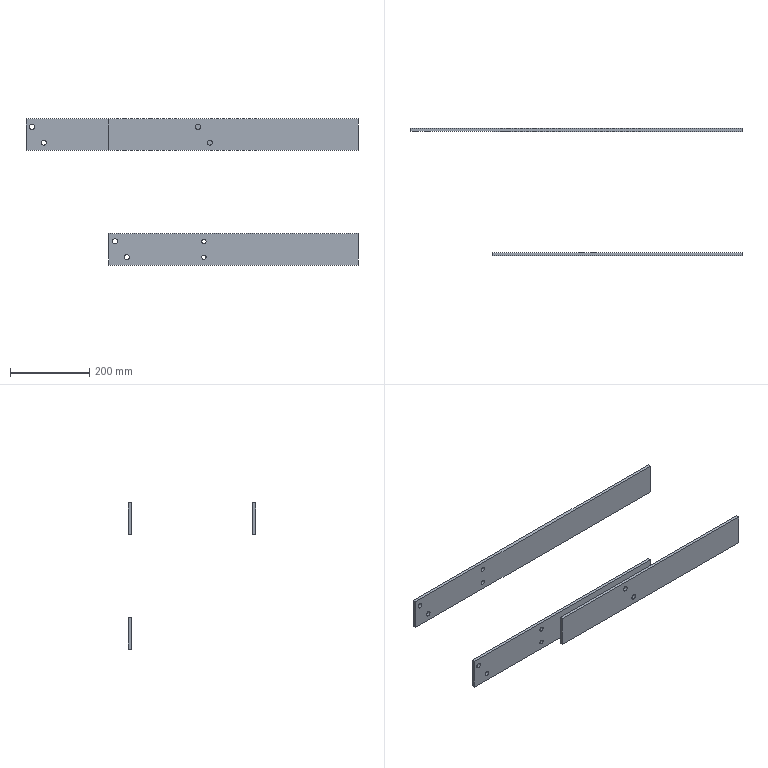Part | SolidWorks | features BaseBody 3 | 3 solids | 38 faces | box 840 x 323 x 370 mm | volume 1334588 mm3 | cylinder 20 | plane 18 | commonest cylinder face diameters 13 x12 11 x8
STEP:
#1=CARTESIAN_POINT('',(561.946,-3179.473,1586.471));
#2=VERTEX_POINT('',#1);
#3=CARTESIAN_POINT('',(561.946,-3179.473,1573.471));
#4=VERTEX_POINT('',#3);
#5=CARTESIAN_POINT('',(561.946,-3179.473,1579.971));
#6=DIRECTION('',(0.,-1.,0.));
#7=DIRECTION('',(0.,0.,-1.));
#8=AXIS2_PLACEMENT_3D('',#5,#6,#7);
#9=CIRCLE('',#8,6.5);
#10=EDGE_CURVE('',#2,#4,#9,.T.);
#11=ORIENTED_EDGE('',*,*,#10,.F.);
#12=CARTESIAN_POINT('',(561.946,-3187.473,1586.471));
#13=VERTEX_POINT('',#12);
#14=CARTESIAN_POINT('',(561.946,-3170.754,1586.471));
#15=DIRECTION('',(0.,-1.,0.));
#16=VECTOR('',#15,1000.);
#17=LINE('',#14,#16);
#18=EDGE_CURVE('',#2,#13,#17,.T.);
#19=ORIENTED_EDGE('',*,*,#18,.T.);
#20=CARTESIAN_POINT('',(561.946,-3187.473,1573.471));
#21=VERTEX_POINT('',#20);
#22=CARTESIAN_POINT('',(561.946,-3187.473,1579.971));
#23=DIRECTION('',(0.,1.,0.));
#24=DIRECTION('',(0.,0.,-1.));
#25=AXIS2_PLACEMENT_3D('',#22,#23,#24);
#26=CIRCLE('',#25,6.5);
#27=EDGE_CURVE('',#21,#13,#26,.T.);
#28=ORIENTED_EDGE('',*,*,#27,.F.);
#29=CARTESIAN_POINT('',(561.946,-3170.754,1573.471));
#30=DIRECTION('',(0.,-1.,0.));
#31=VECTOR('',#30,1000.);
#32=LINE('',#29,#31);
#33=EDGE_CURVE('',#4,#21,#32,.T.);
#34=ORIENTED_EDGE('',*,*,#33,.F.);
#35=EDGE_LOOP('',(#11,#19,#28,#34));
#36=FACE_OUTER_BOUND('',#35,.T.);
#37=CARTESIAN_POINT('',(561.946,-3170.754,1579.971));
#38=DIRECTION('',(0.,-1.,0.));
#39=DIRECTION('',(0.,0.,-1.));
#40=AXIS2_PLACEMENT_3D('',#37,#38,#39);
#41=CYLINDRICAL_SURFACE('',#40,6.5);
#42=ADVANCED_FACE('',(#36),#41,.F.);
#43=CARTESIAN_POINT('',(531.946,-3179.473,1626.471));
#44=VERTEX_POINT('',#43);
#45=CARTESIAN_POINT('',(531.946,-3179.473,1613.471));
#46=VERTEX_POINT('',#45);
#47=CARTESIAN_POINT('',(531.946,-3179.473,1619.971));
#48=DIRECTION('',(0.,-1.,0.));
#49=DIRECTION('',(0.,0.,-1.));
#50=AXIS2_PLACEMENT_3D('',#47,#48,#49);
#51=CIRCLE('',#50,6.5);
#52=EDGE_CURVE('',#44,#46,#51,.T.);
#53=ORIENTED_EDGE('',*,*,#52,.F.);
#54=CARTESIAN_POINT('',(531.946,-3187.473,1626.471));
#55=VERTEX_POINT('',#54);
#56=CARTESIAN_POINT('',(531.946,-3184.932,1626.471));
#57=DIRECTION('',(0.,-1.,0.));
#58=VECTOR('',#57,1000.);
#59=LINE('',#56,#58);
#60=EDGE_CURVE('',#44,#55,#59,.T.);
#61=ORIENTED_EDGE('',*,*,#60,.T.);
#62=CARTESIAN_POINT('',(531.946,-3187.473,1613.471));
#63=VERTEX_POINT('',#62);
#64=CARTESIAN_POINT('',(531.946,-3187.473,1619.971));
#65=DIRECTION('',(0.,1.,0.));
#66=DIRECTION('',(0.,0.,-1.));
#67=AXIS2_PLACEMENT_3D('',#64,#65,#66);
#68=CIRCLE('',#67,6.5);
#69=EDGE_CURVE('',#63,#55,#68,.T.);
#70=ORIENTED_EDGE('',*,*,#69,.F.);
#71=CARTESIAN_POINT('',(531.946,-3184.932,1613.471));
#72=DIRECTION('',(0.,-1.,0.));
#73=VECTOR('',#72,1000.);
#74=LINE('',#71,#73);
#75=EDGE_CURVE('',#46,#63,#74,.T.);
#76=ORIENTED_EDGE('',*,*,#75,.F.);
#77=EDGE_LOOP('',(#53,#61,#70,#76));
#78=FACE_OUTER_BOUND('',#77,.T.);
#79=CARTESIAN_POINT('',(531.946,-3184.932,1619.971));
#80=DIRECTION('',(0.,-1.,0.));
#81=DIRECTION('',(0.,0.,-1.));
#82=AXIS2_PLACEMENT_3D('',#79,#80,#81);
#83=CYLINDRICAL_SURFACE('',#82,6.5);
#84=ADVANCED_FACE('',(#78),#83,.F.);
#85=CARTESIAN_POINT('',(756.946,-3179.473,1625.471));
#86=VERTEX_POINT('',#85);
#87=CARTESIAN_POINT('',(756.946,-3179.473,1614.471));
#88=VERTEX_POINT('',#87);
#89=CARTESIAN_POINT('',(756.946,-3179.473,1619.971));
#90=DIRECTION('',(0.,-1.,0.));
#91=DIRECTION('',(0.,0.,-1.));
#92=AXIS2_PLACEMENT_3D('',#89,#90,#91);
#93=CIRCLE('',#92,5.5);
#94=EDGE_CURVE('',#86,#88,#93,.T.);
#95=ORIENTED_EDGE('',*,*,#94,.F.);
#96=CARTESIAN_POINT('',(756.946,-3187.473,1625.471));
#97=VERTEX_POINT('',#96);
#98=CARTESIAN_POINT('',(756.946,-3201.519,1625.471));
#99=DIRECTION('',(0.,-1.,0.));
#100=VECTOR('',#99,1000.);
#101=LINE('',#98,#100);
#102=EDGE_CURVE('',#86,#97,#101,.T.);
#103=ORIENTED_EDGE('',*,*,#102,.T.);
#104=CARTESIAN_POINT('',(756.946,-3187.473,1614.471));
#105=VERTEX_POINT('',#104);
#106=CARTESIAN_POINT('',(756.946,-3187.473,1619.971));
#107=DIRECTION('',(0.,1.,0.));
#108=DIRECTION('',(0.,0.,-1.));
#109=AXIS2_PLACEMENT_3D('',#106,#107,#108);
#110=CIRCLE('',#109,5.5);
#111=EDGE_CURVE('',#105,#97,#110,.T.);
#112=ORIENTED_EDGE('',*,*,#111,.F.);
#113=CARTESIAN_POINT('',(756.946,-3201.519,1614.471));
#114=DIRECTION('',(0.,-1.,0.));
#115=VECTOR('',#114,1000.);
#116=LINE('',#113,#115);
#117=EDGE_CURVE('',#88,#105,#116,.T.);
#118=ORIENTED_EDGE('',*,*,#117,.F.);
#119=EDGE_LOOP('',(#95,#103,#112,#118));
#120=FACE_OUTER_BOUND('',#119,.T.);
#121=CARTESIAN_POINT('',(756.946,-3201.519,1619.971));
#122=DIRECTION('',(0.,-1.,0.));
#123=DIRECTION('',(0.,0.,-1.));
#124=AXIS2_PLACEMENT_3D('',#121,#122,#123);
#125=CYLINDRICAL_SURFACE('',#124,5.5);
#126=ADVANCED_FACE('',(#120),#125,.F.);
#127=CARTESIAN_POINT('',(756.946,-3179.473,1585.471));
#128=VERTEX_POINT('',#127);
#129=CARTESIAN_POINT('',(756.946,-3179.473,1574.471));
#130=VERTEX_POINT('',#129);
#131=CARTESIAN_POINT('',(756.946,-3179.473,1579.971));
#132=DIRECTION('',(0.,-1.,0.));
#133=DIRECTION('',(0.,0.,-1.));
#134=AXIS2_PLACEMENT_3D('',#131,#132,#133);
#135=CIRCLE('',#134,5.5);
#136=EDGE_CURVE('',#128,#130,#135,.T.);
#137=ORIENTED_EDGE('',*,*,#136,.F.);
#138=CARTESIAN_POINT('',(756.946,-3187.473,1585.471));
#139=VERTEX_POINT('',#138);
#140=CARTESIAN_POINT('',(756.946,-3201.519,1585.471));
#141=DIRECTION('',(0.,-1.,0.));
#142=VECTOR('',#141,1000.);
#143=LINE('',#140,#142);
#144=EDGE_CURVE('',#128,#139,#143,.T.);
#145=ORIENTED_EDGE('',*,*,#144,.T.);
#146=CARTESIAN_POINT('',(756.946,-3187.473,1574.471));
#147=VERTEX_POINT('',#146);
#148=CARTESIAN_POINT('',(756.946,-3187.473,1579.971));
#149=DIRECTION('',(0.,1.,0.));
#150=DIRECTION('',(0.,0.,-1.));
#151=AXIS2_PLACEMENT_3D('',#148,#149,#150);
#152=CIRCLE('',#151,5.5);
#153=EDGE_CURVE('',#147,#139,#152,.T.);
#154=ORIENTED_EDGE('',*,*,#153,.F.);
#155=CARTESIAN_POINT('',(756.946,-3201.519,1574.471));
#156=DIRECTION('',(0.,-1.,0.));
#157=VECTOR('',#156,1000.);
#158=LINE('',#155,#157);
#159=EDGE_CURVE('',#130,#147,#158,.T.);
#160=ORIENTED_EDGE('',*,*,#159,.F.);
#161=EDGE_LOOP('',(#137,#145,#154,#160));
#162=FACE_OUTER_BOUND('',#161,.T.);
#163=CARTESIAN_POINT('',(756.946,-3201.519,1579.971));
#164=DIRECTION('',(0.,-1.,0.));
#165=DIRECTION('',(0.,0.,-1.));
#166=AXIS2_PLACEMENT_3D('',#163,#164,#165);
#167=CYLINDRICAL_SURFACE('',#166,5.5);
#168=ADVANCED_FACE('',(#162),#167,.F.);
#169=CARTESIAN_POINT('',(561.946,-3179.473,1579.971));
#170=DIRECTION('',(0.,-1.,0.));
#171=DIRECTION('',(0.,0.,-1.));
#172=AXIS2_PLACEMENT_3D('',#169,#170,#171);
#173=CIRCLE('',#172,6.5);
#174=EDGE_CURVE('',#4,#2,#173,.T.);
#175=ORIENTED_EDGE('',*,*,#174,.T.);
#176=ORIENTED_EDGE('',*,*,#10,.T.);
#177=EDGE_LOOP('',(#175,#176));
#178=FACE_BOUND('',#177,.T.);
#179=CARTESIAN_POINT('',(531.946,-3179.473,1619.971));
#180=DIRECTION('',(0.,-1.,0.));
#181=DIRECTION('',(0.,0.,-1.));
#182=AXIS2_PLACEMENT_3D('',#179,#180,#181);
#183=CIRCLE('',#182,6.5);
#184=EDGE_CURVE('',#46,#44,#183,.T.);
#185=ORIENTED_EDGE('',*,*,#184,.T.);
#186=ORIENTED_EDGE('',*,*,#52,.T.);
#187=EDGE_LOOP('',(#185,#186));
#188=FACE_BOUND('',#187,.T.);
#189=CARTESIAN_POINT('',(756.946,-3179.473,1619.971));
#190=DIRECTION('',(0.,-1.,0.));
#191=DIRECTION('',(0.,0.,-1.));
#192=AXIS2_PLACEMENT_3D('',#189,#190,#191);
#193=CIRCLE('',#192,5.5);
#194=EDGE_CURVE('',#88,#86,#193,.T.);
#195=ORIENTED_EDGE('',*,*,#194,.T.);
#196=ORIENTED_EDGE('',*,*,#94,.T.);
#197=EDGE_LOOP('',(#195,#196));
#198=FACE_BOUND('',#197,.T.);
#199=CARTESIAN_POINT('',(756.946,-3179.473,1579.971));
#200=DIRECTION('',(0.,-1.,0.));
#201=DIRECTION('',(0.,0.,-1.));
#202=AXIS2_PLACEMENT_3D('',#199,#200,#201);
#203=CIRCLE('',#202,5.5);
#204=EDGE_CURVE('',#130,#128,#203,.T.);
#205=ORIENTED_EDGE('',*,*,#204,.T.);
#206=ORIENTED_EDGE('',*,*,#136,.T.);
#207=EDGE_LOOP('',(#205,#206));
#208=FACE_BOUND('',#207,.T.);
#209=CARTESIAN_POINT('',(516.946,-3179.473,1559.971));
#210=VERTEX_POINT('',#209);
#211=CARTESIAN_POINT('',(516.946,-3179.473,1639.971));
#212=VERTEX_POINT('',#211);
#213=CARTESIAN_POINT('',(516.946,-3179.473,1544.971));
#214=DIRECTION('',(0.,0.,1.));
#215=VECTOR('',#214,1000.);
#216=LINE('',#213,#215);
#217=EDGE_CURVE('',#210,#212,#216,.T.);
#218=ORIENTED_EDGE('',*,*,#217,.T.);
#219=CARTESIAN_POINT('',(1146.946,-3179.473,1639.971));
#220=VERTEX_POINT('',#219);
#221=CARTESIAN_POINT('',(1516.946,-3179.473,1639.971));
#222=DIRECTION('',(1.,0.,0.));
#223=VECTOR('',#222,1000.);
#224=LINE('',#221,#223);
#225=EDGE_CURVE('',#212,#220,#224,.T.);
#226=ORIENTED_EDGE('',*,*,#225,.T.);
#227=CARTESIAN_POINT('',(1146.946,-3179.473,1559.971));
#228=VERTEX_POINT('',#227);
#229=CARTESIAN_POINT('',(1146.946,-3179.473,1544.971));
#230=DIRECTION('',(0.,0.,-1.));
#231=VECTOR('',#230,1000.);
#232=LINE('',#229,#231);
#233=EDGE_CURVE('',#220,#228,#232,.T.);
#234=ORIENTED_EDGE('',*,*,#233,.T.);
#235=CARTESIAN_POINT('',(1516.946,-3179.473,1559.971));
#236=DIRECTION('',(-1.,0.,0.));
#237=VECTOR('',#236,1000.);
#238=LINE('',#235,#237);
#239=EDGE_CURVE('',#228,#210,#238,.T.);
#240=ORIENTED_EDGE('',*,*,#239,.T.);
#241=EDGE_LOOP('',(#218,#226,#234,#240));
#242=FACE_OUTER_BOUND('',#241,.T.);
#243=CARTESIAN_POINT('',(1516.946,-3179.473,1544.971));
#244=DIRECTION('',(0.,1.,0.));
#245=DIRECTION('',(0.,0.,1.));
#246=AXIS2_PLACEMENT_3D('',#243,#244,#245);
#247=PLANE('',#246);
#248=ADVANCED_FACE('',(#178,#188,#198,#208,#242),#247,.T.);
#249=ORIENTED_EDGE('',*,*,#18,.F.);
#250=ORIENTED_EDGE('',*,*,#174,.F.);
#251=ORIENTED_EDGE('',*,*,#33,.T.);
#252=CARTESIAN_POINT('',(561.946,-3187.473,1579.971));
#253=DIRECTION('',(0.,1.,0.));
#254=DIRECTION('',(0.,0.,-1.));
#255=AXIS2_PLACEMENT_3D('',#252,#253,#254);
#256=CIRCLE('',#255,6.5);
#257=EDGE_CURVE('',#13,#21,#256,.T.);
#258=ORIENTED_EDGE('',*,*,#257,.F.);
#259=EDGE_LOOP('',(#249,#250,#251,#258));
#260=FACE_OUTER_BOUND('',#259,.T.);
#261=CARTESIAN_POINT('',(561.946,-3170.754,1579.971));
#262=DIRECTION('',(0.,-1.,0.));
#263=DIRECTION('',(0.,0.,-1.));
#264=AXIS2_PLACEMENT_3D('',#261,#262,#263);
#265=CYLINDRICAL_SURFACE('',#264,6.5);
#266=ADVANCED_FACE('',(#260),#265,.F.);
#267=ORIENTED_EDGE('',*,*,#60,.F.);
#268=ORIENTED_EDGE('',*,*,#184,.F.);
#269=ORIENTED_EDGE('',*,*,#75,.T.);
#270=CARTESIAN_POINT('',(531.946,-3187.473,1619.971));
#271=DIRECTION('',(0.,1.,0.));
#272=DIRECTION('',(0.,0.,-1.));
#273=AXIS2_PLACEMENT_3D('',#270,#271,#272);
#274=CIRCLE('',#273,6.5);
#275=EDGE_CURVE('',#55,#63,#274,.T.);
#276=ORIENTED_EDGE('',*,*,#275,.F.);
#277=EDGE_LOOP('',(#267,#268,#269,#276));
#278=FACE_OUTER_BOUND('',#277,.T.);
#279=CARTESIAN_POINT('',(531.946,-3184.932,1619.971));
#280=DIRECTION('',(0.,-1.,0.));
#281=DIRECTION('',(0.,0.,-1.));
#282=AXIS2_PLACEMENT_3D('',#279,#280,#281);
#283=CYLINDRICAL_SURFACE('',#282,6.5);
#284=ADVANCED_FACE('',(#278),#283,.F.);
#285=ORIENTED_EDGE('',*,*,#102,.F.);
#286=ORIENTED_EDGE('',*,*,#194,.F.);
#287=ORIENTED_EDGE('',*,*,#117,.T.);
#288=CARTESIAN_POINT('',(756.946,-3187.473,1619.971));
#289=DIRECTION('',(0.,1.,0.));
#290=DIRECTION('',(0.,0.,-1.));
#291=AXIS2_PLACEMENT_3D('',#288,#289,#290);
#292=CIRCLE('',#291,5.5);
#293=EDGE_CURVE('',#97,#105,#292,.T.);
#294=ORIENTED_EDGE('',*,*,#293,.F.);
#295=EDGE_LOOP('',(#285,#286,#287,#294));
#296=FACE_OUTER_BOUND('',#295,.T.);
#297=CARTESIAN_POINT('',(756.946,-3201.519,1619.971));
#298=DIRECTION('',(0.,-1.,0.));
#299=DIRECTION('',(0.,0.,-1.));
#300=AXIS2_PLACEMENT_3D('',#297,#298,#299);
#301=CYLINDRICAL_SURFACE('',#300,5.5);
#302=ADVANCED_FACE('',(#296),#301,.F.);
#303=ORIENTED_EDGE('',*,*,#144,.F.);
#304=ORIENTED_EDGE('',*,*,#204,.F.);
#305=ORIENTED_EDGE('',*,*,#159,.T.);
#306=CARTESIAN_POINT('',(756.946,-3187.473,1579.971));
#307=DIRECTION('',(0.,1.,0.));
#308=DIRECTION('',(0.,0.,-1.));
#309=AXIS2_PLACEMENT_3D('',#306,#307,#308);
#310=CIRCLE('',#309,5.5);
#311=EDGE_CURVE('',#139,#147,#310,.T.);
#312=ORIENTED_EDGE('',*,*,#311,.F.);
#313=EDGE_LOOP('',(#303,#304,#305,#312));
#314=FACE_OUTER_BOUND('',#313,.T.);
#315=CARTESIAN_POINT('',(756.946,-3201.519,1579.971));
#316=DIRECTION('',(0.,-1.,0.));
#317=DIRECTION('',(0.,0.,-1.));
#318=AXIS2_PLACEMENT_3D('',#315,#316,#317);
#319=CYLINDRICAL_SURFACE('',#318,5.5);
#320=ADVANCED_FACE('',(#314),#319,.F.);
#321=CARTESIAN_POINT('',(516.946,-3187.473,1639.971));
#322=VERTEX_POINT('',#321);
#323=CARTESIAN_POINT('',(516.946,-3179.473,1639.971));
#324=DIRECTION('',(0.,-1.,0.));
#325=VECTOR('',#324,1000.);
#326=LINE('',#323,#325);
#327=EDGE_CURVE('',#212,#322,#326,.T.);
#328=ORIENTED_EDGE('',*,*,#327,.T.);
#329=CARTESIAN_POINT('',(1146.946,-3187.473,1639.971));
#330=VERTEX_POINT('',#329);
#331=CARTESIAN_POINT('',(1516.946,-3187.473,1639.971));
#332=DIRECTION('',(1.,0.,0.));
#333=VECTOR('',#332,1000.);
#334=LINE('',#331,#333);
#335=EDGE_CURVE('',#322,#330,#334,.T.);
#336=ORIENTED_EDGE('',*,*,#335,.T.);
#337=CARTESIAN_POINT('',(1146.946,-3179.473,1639.971));
#338=DIRECTION('',(0.,1.,0.));
#339=VECTOR('',#338,1000.);
#340=LINE('',#337,#339);
#341=EDGE_CURVE('',#330,#220,#340,.T.);
#342=ORIENTED_EDGE('',*,*,#341,.T.);
#343=ORIENTED_EDGE('',*,*,#225,.F.);
#344=EDGE_LOOP('',(#328,#336,#342,#343));
#345=FACE_OUTER_BOUND('',#344,.T.);
#346=CARTESIAN_POINT('',(1516.946,-3179.473,1639.971));
#347=DIRECTION('',(0.,0.,1.));
#348=DIRECTION('',(1.,0.,0.));
#349=AXIS2_PLACEMENT_3D('',#346,#347,#348);
#350=PLANE('',#349);
#351=ADVANCED_FACE('',(#345),#350,.T.);
#352=CARTESIAN_POINT('',(516.946,-3187.473,1559.971));
#353=VERTEX_POINT('',#352);
#354=CARTESIAN_POINT('',(516.946,-3183.473,1559.971));
#355=DIRECTION('',(0.,1.,0.));
#356=VECTOR('',#355,1000.);
#357=LINE('',#354,#356);
#358=EDGE_CURVE('',#353,#210,#357,.T.);
#359=ORIENTED_EDGE('',*,*,#358,.F.);
#360=CARTESIAN_POINT('',(516.946,-3187.473,1599.971));
#361=DIRECTION('',(0.,0.,-1.));
#362=VECTOR('',#361,1000.);
#363=LINE('',#360,#362);
#364=EDGE_CURVE('',#322,#353,#363,.T.);
#365=ORIENTED_EDGE('',*,*,#364,.F.);
#366=ORIENTED_EDGE('',*,*,#327,.F.);
#367=ORIENTED_EDGE('',*,*,#217,.F.);
#368=EDGE_LOOP('',(#359,#365,#366,#367));
#369=FACE_OUTER_BOUND('',#368,.T.);
#370=CARTESIAN_POINT('',(516.946,-3183.473,1599.971));
#371=DIRECTION('',(1.,0.,0.));
#372=DIRECTION('',(0.,0.,-1.));
#373=AXIS2_PLACEMENT_3D('',#370,#371,#372);
#374=PLANE('',#373);
#375=ADVANCED_FACE('',(#369),#374,.F.);
#376=ORIENTED_EDGE('',*,*,#358,.T.);
#377=ORIENTED_EDGE('',*,*,#239,.F.);
#378=CARTESIAN_POINT('',(1146.946,-3187.473,1559.971));
#379=VERTEX_POINT('',#378);
#380=CARTESIAN_POINT('',(1146.946,-3187.473,1559.971));
#381=DIRECTION('',(0.,-1.,0.));
#382=VECTOR('',#381,1000.);
#383=LINE('',#380,#382);
#384=EDGE_CURVE('',#228,#379,#383,.T.);
#385=ORIENTED_EDGE('',*,*,#384,.T.);
#386=CARTESIAN_POINT('',(1516.946,-3187.473,1559.971));
#387=DIRECTION('',(-1.,0.,0.));
#388=VECTOR('',#387,1000.);
#389=LINE('',#386,#388);
#390=EDGE_CURVE('',#379,#353,#389,.T.);
#391=ORIENTED_EDGE('',*,*,#390,.T.);
#392=EDGE_LOOP('',(#376,#377,#385,#391));
#393=FACE_OUTER_BOUND('',#392,.T.);
#394=CARTESIAN_POINT('',(1516.946,-3187.473,1559.971));
#395=DIRECTION('',(0.,0.,-1.));
#396=DIRECTION('',(-1.,0.,0.));
#397=AXIS2_PLACEMENT_3D('',#394,#395,#396);
#398=PLANE('',#397);
#399=ADVANCED_FACE('',(#393),#398,.T.);
#400=ORIENTED_EDGE('',*,*,#341,.F.);
#401=CARTESIAN_POINT('',(1146.946,-3187.473,1262.326));
#402=DIRECTION('',(0.,0.,1.));
#403=VECTOR('',#402,1000.);
#404=LINE('',#401,#403);
#405=EDGE_CURVE('',#379,#330,#404,.T.);
#406=ORIENTED_EDGE('',*,*,#405,.F.);
#407=ORIENTED_EDGE('',*,*,#384,.F.);
#408=ORIENTED_EDGE('',*,*,#233,.F.);
#409=EDGE_LOOP('',(#400,#406,#407,#408));
#410=FACE_OUTER_BOUND('',#409,.T.);
#411=CARTESIAN_POINT('',(1146.946,-2903.218,1262.326));
#412=DIRECTION('',(-1.,0.,0.));
#413=DIRECTION('',(0.,0.,1.));
#414=AXIS2_PLACEMENT_3D('',#411,#412,#413);
#415=PLANE('',#414);
#416=ADVANCED_FACE('',(#410),#415,.F.);
#417=ORIENTED_EDGE('',*,*,#153,.T.);
#418=ORIENTED_EDGE('',*,*,#311,.T.);
#419=EDGE_LOOP('',(#417,#418));
#420=FACE_BOUND('',#419,.T.);
#421=ORIENTED_EDGE('',*,*,#111,.T.);
#422=ORIENTED_EDGE('',*,*,#293,.T.);
#423=EDGE_LOOP('',(#421,#422));
#424=FACE_BOUND('',#423,.T.);
#425=ORIENTED_EDGE('',*,*,#69,.T.);
#426=ORIENTED_EDGE('',*,*,#275,.T.);
#427=EDGE_LOOP('',(#425,#426));
#428=FACE_BOUND('',#427,.T.);
#429=ORIENTED_EDGE('',*,*,#27,.T.);
#430=ORIENTED_EDGE('',*,*,#257,.T.);
#431=EDGE_LOOP('',(#429,#430));
#432=FACE_BOUND('',#431,.T.);
#433=ORIENTED_EDGE('',*,*,#364,.T.);
#434=ORIENTED_EDGE('',*,*,#390,.F.);
#435=ORIENTED_EDGE('',*,*,#405,.T.);
#436=ORIENTED_EDGE('',*,*,#335,.F.);
#437=EDGE_LOOP('',(#433,#434,#435,#436));
#438=FACE_OUTER_BOUND('',#437,.T.);
#439=CARTESIAN_POINT('',(1516.946,-3187.473,1639.971));
#440=DIRECTION('',(0.,-1.,0.));
#441=DIRECTION('',(0.,0.,-1.));
#442=AXIS2_PLACEMENT_3D('',#439,#440,#441);
#443=PLANE('',#442);
#444=ADVANCED_FACE('',(#420,#424,#428,#432,#438),#443,.T.);
#445=CLOSED_SHELL('',(#42,#84,#126,#168,#248,#266,#284,#302,#320,#351,#375,#399,#416,#444));
#446=MANIFOLD_SOLID_BREP('',#445);
#447=CARTESIAN_POINT('',(741.946,-3494.473,1916.471));
#448=VERTEX_POINT('',#447);
#449=CARTESIAN_POINT('',(741.946,-3494.473,1903.471));
#450=VERTEX_POINT('',#449);
#451=CARTESIAN_POINT('',(741.946,-3494.473,1909.971));
#452=DIRECTION('',(0.,-1.,0.));
#453=DIRECTION('',(0.,0.,-1.));
#454=AXIS2_PLACEMENT_3D('',#451,#452,#453);
#455=CIRCLE('',#454,6.5);
#456=EDGE_CURVE('',#448,#450,#455,.T.);
#457=ORIENTED_EDGE('',*,*,#456,.F.);
#458=CARTESIAN_POINT('',(741.946,-3502.473,1916.471));
#459=VERTEX_POINT('',#458);
#460=CARTESIAN_POINT('',(741.946,-3516.007,1916.471));
#461=DIRECTION('',(0.,-1.,0.));
#462=VECTOR('',#461,1000.);
#463=LINE('',#460,#462);
#464=EDGE_CURVE('',#448,#459,#463,.T.);
#465=ORIENTED_EDGE('',*,*,#464,.T.);
#466=CARTESIAN_POINT('',(741.946,-3502.473,1903.471));
#467=VERTEX_POINT('',#466);
#468=CARTESIAN_POINT('',(741.946,-3502.473,1909.971));
#469=DIRECTION('',(0.,1.,0.));
#470=DIRECTION('',(0.,0.,-1.));
#471=AXIS2_PLACEMENT_3D('',#468,#469,#470);
#472=CIRCLE('',#471,6.5);
#473=EDGE_CURVE('',#467,#459,#472,.T.);
#474=ORIENTED_EDGE('',*,*,#473,.F.);
#475=CARTESIAN_POINT('',(741.946,-3516.007,1903.471));
#476=DIRECTION('',(0.,-1.,0.));
#477=VECTOR('',#476,1000.);
#478=LINE('',#475,#477);
#479=EDGE_CURVE('',#450,#467,#478,.T.);
#480=ORIENTED_EDGE('',*,*,#479,.F.);
#481=EDGE_LOOP('',(#457,#465,#474,#480));
#482=FACE_OUTER_BOUND('',#481,.T.);
#483=CARTESIAN_POINT('',(741.946,-3516.007,1909.971));
#484=DIRECTION('',(0.,-1.,0.));
#485=DIRECTION('',(0.,0.,-1.));
#486=AXIS2_PLACEMENT_3D('',#483,#484,#485);
#487=CYLINDRICAL_SURFACE('',#486,6.5);
#488=ADVANCED_FACE('',(#482),#487,.F.);
#489=CARTESIAN_POINT('',(771.946,-3494.473,1876.471));
#490=VERTEX_POINT('',#489);
#491=CARTESIAN_POINT('',(771.946,-3494.473,1863.471));
#492=VERTEX_POINT('',#491);
#493=CARTESIAN_POINT('',(771.946,-3494.473,1869.971));
#494=DIRECTION('',(0.,-1.,0.));
#495=DIRECTION('',(0.,0.,-1.));
#496=AXIS2_PLACEMENT_3D('',#493,#494,#495);
#497=CIRCLE('',#496,6.5);
#498=EDGE_CURVE('',#490,#492,#497,.T.);
#499=ORIENTED_EDGE('',*,*,#498,.F.);
#500=CARTESIAN_POINT('',(771.946,-3502.473,1876.471));
#501=VERTEX_POINT('',#500);
#502=CARTESIAN_POINT('',(771.946,-3513.416,1876.471));
#503=DIRECTION('',(0.,-1.,0.));
#504=VECTOR('',#503,1000.);
#505=LINE('',#502,#504);
#506=EDGE_CURVE('',#490,#501,#505,.T.);
#507=ORIENTED_EDGE('',*,*,#506,.T.);
#508=CARTESIAN_POINT('',(771.946,-3502.473,1863.471));
#509=VERTEX_POINT('',#508);
#510=CARTESIAN_POINT('',(771.946,-3502.473,1869.971));
#511=DIRECTION('',(0.,1.,0.));
#512=DIRECTION('',(0.,0.,-1.));
#513=AXIS2_PLACEMENT_3D('',#510,#511,#512);
#514=CIRCLE('',#513,6.5);
#515=EDGE_CURVE('',#509,#501,#514,.T.);
#516=ORIENTED_EDGE('',*,*,#515,.F.);
#517=CARTESIAN_POINT('',(771.946,-3513.416,1863.471));
#518=DIRECTION('',(0.,-1.,0.));
#519=VECTOR('',#518,1000.);
#520=LINE('',#517,#519);
#521=EDGE_CURVE('',#492,#509,#520,.T.);
#522=ORIENTED_EDGE('',*,*,#521,.F.);
#523=EDGE_LOOP('',(#499,#507,#516,#522));
#524=FACE_OUTER_BOUND('',#523,.T.);
#525=CARTESIAN_POINT('',(771.946,-3513.416,1869.971));
#526=DIRECTION('',(0.,-1.,0.));
#527=DIRECTION('',(0.,0.,-1.));
#528=AXIS2_PLACEMENT_3D('',#525,#526,#527);
#529=CYLINDRICAL_SURFACE('',#528,6.5);
#530=ADVANCED_FACE('',(#524),#529,.F.);
#531=ORIENTED_EDGE('',*,*,#473,.T.);
#532=CARTESIAN_POINT('',(741.946,-3502.473,1909.971));
#533=DIRECTION('',(0.,1.,0.));
#534=DIRECTION('',(0.,0.,-1.));
#535=AXIS2_PLACEMENT_3D('',#532,#533,#534);
#536=CIRCLE('',#535,6.5);
#537=EDGE_CURVE('',#459,#467,#536,.T.);
#538=ORIENTED_EDGE('',*,*,#537,.T.);
#539=EDGE_LOOP('',(#531,#538));
#540=FACE_BOUND('',#539,.T.);
#541=ORIENTED_EDGE('',*,*,#515,.T.);
#542=CARTESIAN_POINT('',(771.946,-3502.473,1869.971));
#543=DIRECTION('',(0.,1.,0.));
#544=DIRECTION('',(0.,0.,-1.));
#545=AXIS2_PLACEMENT_3D('',#542,#543,#544);
#546=CIRCLE('',#545,6.5);
#547=EDGE_CURVE('',#501,#509,#546,.T.);
#548=ORIENTED_EDGE('',*,*,#547,.T.);
#549=EDGE_LOOP('',(#541,#548));
#550=FACE_BOUND('',#549,.T.);
#551=CARTESIAN_POINT('',(516.946,-3502.473,1929.971));
#552=VERTEX_POINT('',#551);
#553=CARTESIAN_POINT('',(516.946,-3502.473,1849.971));
#554=VERTEX_POINT('',#553);
#555=CARTESIAN_POINT('',(516.946,-3502.473,1929.971));
#556=DIRECTION('',(0.,0.,-1.));
#557=VECTOR('',#556,1000.);
#558=LINE('',#555,#557);
#559=EDGE_CURVE('',#552,#554,#558,.T.);
#560=ORIENTED_EDGE('',*,*,#559,.T.);
#561=CARTESIAN_POINT('',(1146.946,-3502.473,1849.971));
#562=VERTEX_POINT('',#561);
#563=CARTESIAN_POINT('',(1516.946,-3502.473,1849.971));
#564=DIRECTION('',(1.,0.,0.));
#565=VECTOR('',#564,1000.);
#566=LINE('',#563,#565);
#567=EDGE_CURVE('',#554,#562,#566,.T.);
#568=ORIENTED_EDGE('',*,*,#567,.T.);
#569=CARTESIAN_POINT('',(1146.946,-3502.473,1929.971));
#570=VERTEX_POINT('',#569);
#571=CARTESIAN_POINT('',(1146.946,-3502.473,1929.971));
#572=DIRECTION('',(0.,0.,1.));
#573=VECTOR('',#572,1000.);
#574=LINE('',#571,#573);
#575=EDGE_CURVE('',#562,#570,#574,.T.);
#576=ORIENTED_EDGE('',*,*,#575,.T.);
#577=CARTESIAN_POINT('',(1516.946,-3502.473,1929.971));
#578=DIRECTION('',(-1.,0.,0.));
#579=VECTOR('',#578,1000.);
#580=LINE('',#577,#579);
#581=EDGE_CURVE('',#570,#552,#580,.T.);
#582=ORIENTED_EDGE('',*,*,#581,.T.);
#583=EDGE_LOOP('',(#560,#568,#576,#582));
#584=FACE_OUTER_BOUND('',#583,.T.);
#585=CARTESIAN_POINT('',(1516.946,-3502.473,1929.971));
#586=DIRECTION('',(0.,-1.,0.));
#587=DIRECTION('',(0.,0.,-1.));
#588=AXIS2_PLACEMENT_3D('',#585,#586,#587);
#589=PLANE('',#588);
#590=ADVANCED_FACE('',(#540,#550,#584),#589,.T.);
#591=ORIENTED_EDGE('',*,*,#464,.F.);
#592=CARTESIAN_POINT('',(741.946,-3494.473,1909.971));
#593=DIRECTION('',(0.,-1.,0.));
#594=DIRECTION('',(0.,0.,-1.));
#595=AXIS2_PLACEMENT_3D('',#592,#593,#594);
#596=CIRCLE('',#595,6.5);
#597=EDGE_CURVE('',#450,#448,#596,.T.);
#598=ORIENTED_EDGE('',*,*,#597,.F.);
#599=ORIENTED_EDGE('',*,*,#479,.T.);
#600=ORIENTED_EDGE('',*,*,#537,.F.);
#601=EDGE_LOOP('',(#591,#598,#599,#600));
#602=FACE_OUTER_BOUND('',#601,.T.);
#603=CARTESIAN_POINT('',(741.946,-3516.007,1909.971));
#604=DIRECTION('',(0.,-1.,0.));
#605=DIRECTION('',(0.,0.,-1.));
#606=AXIS2_PLACEMENT_3D('',#603,#604,#605);
#607=CYLINDRICAL_SURFACE('',#606,6.5);
#608=ADVANCED_FACE('',(#602),#607,.F.);
#609=ORIENTED_EDGE('',*,*,#506,.F.);
#610=CARTESIAN_POINT('',(771.946,-3494.473,1869.971));
#611=DIRECTION('',(0.,-1.,0.));
#612=DIRECTION('',(0.,0.,-1.));
#613=AXIS2_PLACEMENT_3D('',#610,#611,#612);
#614=CIRCLE('',#613,6.5);
#615=EDGE_CURVE('',#492,#490,#614,.T.);
#616=ORIENTED_EDGE('',*,*,#615,.F.);
#617=ORIENTED_EDGE('',*,*,#521,.T.);
#618=ORIENTED_EDGE('',*,*,#547,.F.);
#619=EDGE_LOOP('',(#609,#616,#617,#618));
#620=FACE_OUTER_BOUND('',#619,.T.);
#621=CARTESIAN_POINT('',(771.946,-3513.416,1869.971));
#622=DIRECTION('',(0.,-1.,0.));
#623=DIRECTION('',(0.,0.,-1.));
#624=AXIS2_PLACEMENT_3D('',#621,#622,#623);
#625=CYLINDRICAL_SURFACE('',#624,6.5);
#626=ADVANCED_FACE('',(#620),#625,.F.);
#627=CARTESIAN_POINT('',(516.946,-3494.473,1849.971));
#628=VERTEX_POINT('',#627);
#629=CARTESIAN_POINT('',(516.946,-3502.473,1849.971));
#630=DIRECTION('',(0.,1.,0.));
#631=VECTOR('',#630,1000.);
#632=LINE('',#629,#631);
#633=EDGE_CURVE('',#554,#628,#632,.T.);
#634=ORIENTED_EDGE('',*,*,#633,.T.);
#635=CARTESIAN_POINT('',(1146.946,-3494.473,1849.971));
#636=VERTEX_POINT('',#635);
#637=CARTESIAN_POINT('',(1516.946,-3494.473,1849.971));
#638=DIRECTION('',(1.,0.,0.));
#639=VECTOR('',#638,1000.);
#640=LINE('',#637,#639);
#641=EDGE_CURVE('',#628,#636,#640,.T.);
#642=ORIENTED_EDGE('',*,*,#641,.T.);
#643=CARTESIAN_POINT('',(1146.946,-3502.473,1849.971));
#644=DIRECTION('',(0.,-1.,0.));
#645=VECTOR('',#644,1000.);
#646=LINE('',#643,#645);
#647=EDGE_CURVE('',#636,#562,#646,.T.);
#648=ORIENTED_EDGE('',*,*,#647,.T.);
#649=ORIENTED_EDGE('',*,*,#567,.F.);
#650=EDGE_LOOP('',(#634,#642,#648,#649));
#651=FACE_OUTER_BOUND('',#650,.T.);
#652=CARTESIAN_POINT('',(1516.946,-3502.473,1849.971));
#653=DIRECTION('',(0.,0.,-1.));
#654=DIRECTION('',(-1.,0.,0.));
#655=AXIS2_PLACEMENT_3D('',#652,#653,#654);
#656=PLANE('',#655);
#657=ADVANCED_FACE('',(#651),#656,.T.);
#658=ORIENTED_EDGE('',*,*,#633,.F.);
#659=ORIENTED_EDGE('',*,*,#559,.F.);
#660=CARTESIAN_POINT('',(516.946,-3494.473,1929.971));
#661=VERTEX_POINT('',#660);
#662=CARTESIAN_POINT('',(516.946,-3498.473,1929.971));
#663=DIRECTION('',(0.,-1.,0.));
#664=VECTOR('',#663,1000.);
#665=LINE('',#662,#664);
#666=EDGE_CURVE('',#661,#552,#665,.T.);
#667=ORIENTED_EDGE('',*,*,#666,.F.);
#668=CARTESIAN_POINT('',(516.946,-3494.473,1889.971));
#669=DIRECTION('',(0.,0.,1.));
#670=VECTOR('',#669,1000.);
#671=LINE('',#668,#670);
#672=EDGE_CURVE('',#628,#661,#671,.T.);
#673=ORIENTED_EDGE('',*,*,#672,.F.);
#674=EDGE_LOOP('',(#658,#659,#667,#673));
#675=FACE_OUTER_BOUND('',#674,.T.);
#676=CARTESIAN_POINT('',(516.946,-3498.473,1889.971));
#677=DIRECTION('',(1.,0.,0.));
#678=DIRECTION('',(0.,0.,-1.));
#679=AXIS2_PLACEMENT_3D('',#676,#677,#678);
#680=PLANE('',#679);
#681=ADVANCED_FACE('',(#675),#680,.F.);
#682=ORIENTED_EDGE('',*,*,#666,.T.);
#683=ORIENTED_EDGE('',*,*,#581,.F.);
#684=CARTESIAN_POINT('',(1146.946,-3494.473,1929.971));
#685=VERTEX_POINT('',#684);
#686=CARTESIAN_POINT('',(1146.946,-3494.473,1929.971));
#687=DIRECTION('',(0.,1.,0.));
#688=VECTOR('',#687,1000.);
#689=LINE('',#686,#688);
#690=EDGE_CURVE('',#570,#685,#689,.T.);
#691=ORIENTED_EDGE('',*,*,#690,.T.);
#692=CARTESIAN_POINT('',(1516.946,-3494.473,1929.971));
#693=DIRECTION('',(-1.,0.,0.));
#694=VECTOR('',#693,1000.);
#695=LINE('',#692,#694);
#696=EDGE_CURVE('',#685,#661,#695,.T.);
#697=ORIENTED_EDGE('',*,*,#696,.T.);
#698=EDGE_LOOP('',(#682,#683,#691,#697));
#699=FACE_OUTER_BOUND('',#698,.T.);
#700=CARTESIAN_POINT('',(1516.946,-3494.473,1929.971));
#701=DIRECTION('',(0.,0.,1.));
#702=DIRECTION('',(1.,0.,0.));
#703=AXIS2_PLACEMENT_3D('',#700,#701,#702);
#704=PLANE('',#703);
#705=ADVANCED_FACE('',(#699),#704,.T.);
#706=ORIENTED_EDGE('',*,*,#690,.F.);
#707=ORIENTED_EDGE('',*,*,#575,.F.);
#708=ORIENTED_EDGE('',*,*,#647,.F.);
#709=CARTESIAN_POINT('',(1146.946,-3494.473,1287.326));
#710=DIRECTION('',(0.,0.,-1.));
#711=VECTOR('',#710,1000.);
#712=LINE('',#709,#711);
#713=EDGE_CURVE('',#685,#636,#712,.T.);
#714=ORIENTED_EDGE('',*,*,#713,.F.);
#715=EDGE_LOOP('',(#706,#707,#708,#714));
#716=FACE_OUTER_BOUND('',#715,.T.);
#717=CARTESIAN_POINT('',(1146.946,-2903.218,1287.326));
#718=DIRECTION('',(-1.,0.,0.));
#719=DIRECTION('',(0.,0.,1.));
#720=AXIS2_PLACEMENT_3D('',#717,#718,#719);
#721=PLANE('',#720);
#722=ADVANCED_FACE('',(#716),#721,.F.);
#723=ORIENTED_EDGE('',*,*,#615,.T.);
#724=ORIENTED_EDGE('',*,*,#498,.T.);
#725=EDGE_LOOP('',(#723,#724));
#726=FACE_BOUND('',#725,.T.);
#727=ORIENTED_EDGE('',*,*,#597,.T.);
#728=ORIENTED_EDGE('',*,*,#456,.T.);
#729=EDGE_LOOP('',(#727,#728));
#730=FACE_BOUND('',#729,.T.);
#731=ORIENTED_EDGE('',*,*,#672,.T.);
#732=ORIENTED_EDGE('',*,*,#696,.F.);
#733=ORIENTED_EDGE('',*,*,#713,.T.);
#734=ORIENTED_EDGE('',*,*,#641,.F.);
#735=EDGE_LOOP('',(#731,#732,#733,#734));
#736=FACE_OUTER_BOUND('',#735,.T.);
#737=CARTESIAN_POINT('',(1516.946,-3494.473,1849.971));
#738=DIRECTION('',(0.,1.,0.));
#739=DIRECTION('',(0.,0.,1.));
#740=AXIS2_PLACEMENT_3D('',#737,#738,#739);
#741=PLANE('',#740);
#742=ADVANCED_FACE('',(#726,#730,#736),#741,.T.);
#743=CLOSED_SHELL('',(#488,#530,#590,#608,#626,#657,#681,#705,#722,#742));
#744=MANIFOLD_SOLID_BREP('',#743);
#745=CARTESIAN_POINT('',(546.946,-3179.473,1875.471));
#746=VERTEX_POINT('',#745);
#747=CARTESIAN_POINT('',(546.946,-3179.473,1864.471));
#748=VERTEX_POINT('',#747);
#749=CARTESIAN_POINT('',(546.946,-3179.473,1869.971));
#750=DIRECTION('',(0.,-1.,0.));
#751=DIRECTION('',(0.,0.,-1.));
#752=AXIS2_PLACEMENT_3D('',#749,#750,#751);
#753=CIRCLE('',#752,5.5);
#754=EDGE_CURVE('',#746,#748,#753,.T.);
#755=ORIENTED_EDGE('',*,*,#754,.F.);
#756=CARTESIAN_POINT('',(546.946,-3187.473,1875.471));
#757=VERTEX_POINT('',#756);
#758=CARTESIAN_POINT('',(546.946,-3210.297,1875.471));
#759=DIRECTION('',(0.,-1.,0.));
#760=VECTOR('',#759,1000.);
#761=LINE('',#758,#760);
#762=EDGE_CURVE('',#746,#757,#761,.T.);
#763=ORIENTED_EDGE('',*,*,#762,.T.);
#764=CARTESIAN_POINT('',(546.946,-3187.473,1864.471));
#765=VERTEX_POINT('',#764);
#766=CARTESIAN_POINT('',(546.946,-3187.473,1869.971));
#767=DIRECTION('',(0.,1.,0.));
#768=DIRECTION('',(0.,0.,-1.));
#769=AXIS2_PLACEMENT_3D('',#766,#767,#768);
#770=CIRCLE('',#769,5.5);
#771=EDGE_CURVE('',#765,#757,#770,.T.);
#772=ORIENTED_EDGE('',*,*,#771,.F.);
#773=CARTESIAN_POINT('',(546.946,-3210.297,1864.471));
#774=DIRECTION('',(0.,-1.,0.));
#775=VECTOR('',#774,1000.);
#776=LINE('',#773,#775);
#777=EDGE_CURVE('',#748,#765,#776,.T.);
#778=ORIENTED_EDGE('',*,*,#777,.F.);
#779=EDGE_LOOP('',(#755,#763,#772,#778));
#780=FACE_OUTER_BOUND('',#779,.T.);
#781=CARTESIAN_POINT('',(546.946,-3210.297,1869.971));
#782=DIRECTION('',(0.,-1.,0.));
#783=DIRECTION('',(0.,0.,-1.));
#784=AXIS2_PLACEMENT_3D('',#781,#782,#783);
#785=CYLINDRICAL_SURFACE('',#784,5.5);
#786=ADVANCED_FACE('',(#780),#785,.F.);
#787=CARTESIAN_POINT('',(546.946,-3179.473,1915.471));
#788=VERTEX_POINT('',#787);
#789=CARTESIAN_POINT('',(546.946,-3179.473,1904.471));
#790=VERTEX_POINT('',#789);
#791=CARTESIAN_POINT('',(546.946,-3179.473,1909.971));
#792=DIRECTION('',(0.,-1.,0.));
#793=DIRECTION('',(0.,0.,-1.));
#794=AXIS2_PLACEMENT_3D('',#791,#792,#793);
#795=CIRCLE('',#794,5.5);
#796=EDGE_CURVE('',#788,#790,#795,.T.);
#797=ORIENTED_EDGE('',*,*,#796,.F.);
#798=CARTESIAN_POINT('',(546.946,-3187.473,1915.471));
#799=VERTEX_POINT('',#798);
#800=CARTESIAN_POINT('',(546.946,-3210.297,1915.471));
#801=DIRECTION('',(0.,-1.,0.));
#802=VECTOR('',#801,1000.);
#803=LINE('',#800,#802);
#804=EDGE_CURVE('',#788,#799,#803,.T.);
#805=ORIENTED_EDGE('',*,*,#804,.T.);
#806=CARTESIAN_POINT('',(546.946,-3187.473,1904.471));
#807=VERTEX_POINT('',#806);
#808=CARTESIAN_POINT('',(546.946,-3187.473,1909.971));
#809=DIRECTION('',(0.,1.,0.));
#810=DIRECTION('',(0.,0.,-1.));
#811=AXIS2_PLACEMENT_3D('',#808,#809,#810);
#812=CIRCLE('',#811,5.5);
#813=EDGE_CURVE('',#807,#799,#812,.T.);
#814=ORIENTED_EDGE('',*,*,#813,.F.);
#815=CARTESIAN_POINT('',(546.946,-3210.297,1904.471));
#816=DIRECTION('',(0.,-1.,0.));
#817=VECTOR('',#816,1000.);
#818=LINE('',#815,#817);
#819=EDGE_CURVE('',#790,#807,#818,.T.);
#820=ORIENTED_EDGE('',*,*,#819,.F.);
#821=EDGE_LOOP('',(#797,#805,#814,#820));
#822=FACE_OUTER_BOUND('',#821,.T.);
#823=CARTESIAN_POINT('',(546.946,-3210.297,1909.971));
#824=DIRECTION('',(0.,-1.,0.));
#825=DIRECTION('',(0.,0.,-1.));
#826=AXIS2_PLACEMENT_3D('',#823,#824,#825);
#827=CYLINDRICAL_SURFACE('',#826,5.5);
#828=ADVANCED_FACE('',(#822),#827,.F.);
#829=CARTESIAN_POINT('',(351.946,-3179.473,1876.471));
#830=VERTEX_POINT('',#829);
#831=CARTESIAN_POINT('',(351.946,-3179.473,1863.471));
#832=VERTEX_POINT('',#831);
#833=CARTESIAN_POINT('',(351.946,-3179.473,1869.971));
#834=DIRECTION('',(0.,-1.,0.));
#835=DIRECTION('',(0.,0.,-1.));
#836=AXIS2_PLACEMENT_3D('',#833,#834,#835);
#837=CIRCLE('',#836,6.5);
#838=EDGE_CURVE('',#830,#832,#837,.T.);
#839=ORIENTED_EDGE('',*,*,#838,.F.);
#840=CARTESIAN_POINT('',(351.946,-3187.473,1876.471));
#841=VERTEX_POINT('',#840);
#842=CARTESIAN_POINT('',(351.946,-3160.343,1876.471));
#843=DIRECTION('',(0.,-1.,0.));
#844=VECTOR('',#843,1000.);
#845=LINE('',#842,#844);
#846=EDGE_CURVE('',#830,#841,#845,.T.);
#847=ORIENTED_EDGE('',*,*,#846,.T.);
#848=CARTESIAN_POINT('',(351.946,-3187.473,1863.471));
#849=VERTEX_POINT('',#848);
#850=CARTESIAN_POINT('',(351.946,-3187.473,1869.971));
#851=DIRECTION('',(0.,1.,0.));
#852=DIRECTION('',(0.,0.,-1.));
#853=AXIS2_PLACEMENT_3D('',#850,#851,#852);
#854=CIRCLE('',#853,6.5);
#855=EDGE_CURVE('',#849,#841,#854,.T.);
#856=ORIENTED_EDGE('',*,*,#855,.F.);
#857=CARTESIAN_POINT('',(351.946,-3160.343,1863.471));
#858=DIRECTION('',(0.,-1.,0.));
#859=VECTOR('',#858,1000.);
#860=LINE('',#857,#859);
#861=EDGE_CURVE('',#832,#849,#860,.T.);
#862=ORIENTED_EDGE('',*,*,#861,.F.);
#863=EDGE_LOOP('',(#839,#847,#856,#862));
#864=FACE_OUTER_BOUND('',#863,.T.);
#865=CARTESIAN_POINT('',(351.946,-3160.343,1869.971));
#866=DIRECTION('',(0.,-1.,0.));
#867=DIRECTION('',(0.,0.,-1.));
#868=AXIS2_PLACEMENT_3D('',#865,#866,#867);
#869=CYLINDRICAL_SURFACE('',#868,6.5);
#870=ADVANCED_FACE('',(#864),#869,.F.);
#871=CARTESIAN_POINT('',(321.946,-3179.473,1916.471));
#872=VERTEX_POINT('',#871);
#873=CARTESIAN_POINT('',(321.946,-3179.473,1903.471));
#874=VERTEX_POINT('',#873);
#875=CARTESIAN_POINT('',(321.946,-3179.473,1909.971));
#876=DIRECTION('',(0.,-1.,0.));
#877=DIRECTION('',(0.,0.,-1.));
#878=AXIS2_PLACEMENT_3D('',#875,#876,#877);
#879=CIRCLE('',#878,6.5);
#880=EDGE_CURVE('',#872,#874,#879,.T.);
#881=ORIENTED_EDGE('',*,*,#880,.F.);
#882=CARTESIAN_POINT('',(321.946,-3187.473,1916.471));
#883=VERTEX_POINT('',#882);
#884=CARTESIAN_POINT('',(321.946,-3160.343,1916.471));
#885=DIRECTION('',(0.,-1.,0.));
#886=VECTOR('',#885,1000.);
#887=LINE('',#884,#886);
#888=EDGE_CURVE('',#872,#883,#887,.T.);
#889=ORIENTED_EDGE('',*,*,#888,.T.);
#890=CARTESIAN_POINT('',(321.946,-3187.473,1903.471));
#891=VERTEX_POINT('',#890);
#892=CARTESIAN_POINT('',(321.946,-3187.473,1909.971));
#893=DIRECTION('',(0.,1.,0.));
#894=DIRECTION('',(0.,0.,-1.));
#895=AXIS2_PLACEMENT_3D('',#892,#893,#894);
#896=CIRCLE('',#895,6.5);
#897=EDGE_CURVE('',#891,#883,#896,.T.);
#898=ORIENTED_EDGE('',*,*,#897,.F.);
#899=CARTESIAN_POINT('',(321.946,-3160.343,1903.471));
#900=DIRECTION('',(0.,-1.,0.));
#901=VECTOR('',#900,1000.);
#902=LINE('',#899,#901);
#903=EDGE_CURVE('',#874,#891,#902,.T.);
#904=ORIENTED_EDGE('',*,*,#903,.F.);
#905=EDGE_LOOP('',(#881,#889,#898,#904));
#906=FACE_OUTER_BOUND('',#905,.T.);
#907=CARTESIAN_POINT('',(321.946,-3160.343,1909.971));
#908=DIRECTION('',(0.,-1.,0.));
#909=DIRECTION('',(0.,0.,-1.));
#910=AXIS2_PLACEMENT_3D('',#907,#908,#909);
#911=CYLINDRICAL_SURFACE('',#910,6.5);
#912=ADVANCED_FACE('',(#906),#911,.F.);
#913=ORIENTED_EDGE('',*,*,#771,.T.);
#914=CARTESIAN_POINT('',(546.946,-3187.473,1869.971));
#915=DIRECTION('',(0.,1.,0.));
#916=DIRECTION('',(0.,0.,-1.));
#917=AXIS2_PLACEMENT_3D('',#914,#915,#916);
#918=CIRCLE('',#917,5.5);
#919=EDGE_CURVE('',#757,#765,#918,.T.);
#920=ORIENTED_EDGE('',*,*,#919,.T.);
#921=EDGE_LOOP('',(#913,#920));
#922=FACE_BOUND('',#921,.T.);
#923=ORIENTED_EDGE('',*,*,#813,.T.);
#924=CARTESIAN_POINT('',(546.946,-3187.473,1909.971));
#925=DIRECTION('',(0.,1.,0.));
#926=DIRECTION('',(0.,0.,-1.));
#927=AXIS2_PLACEMENT_3D('',#924,#925,#926);
#928=CIRCLE('',#927,5.5);
#929=EDGE_CURVE('',#799,#807,#928,.T.);
#930=ORIENTED_EDGE('',*,*,#929,.T.);
#931=EDGE_LOOP('',(#923,#930));
#932=FACE_BOUND('',#931,.T.);
#933=ORIENTED_EDGE('',*,*,#855,.T.);
#934=CARTESIAN_POINT('',(351.946,-3187.473,1869.971));
#935=DIRECTION('',(0.,1.,0.));
#936=DIRECTION('',(0.,0.,-1.));
#937=AXIS2_PLACEMENT_3D('',#934,#935,#936);
#938=CIRCLE('',#937,6.5);
#939=EDGE_CURVE('',#841,#849,#938,.T.);
#940=ORIENTED_EDGE('',*,*,#939,.T.);
#941=EDGE_LOOP('',(#933,#940));
#942=FACE_BOUND('',#941,.T.);
#943=ORIENTED_EDGE('',*,*,#897,.T.);
#944=CARTESIAN_POINT('',(321.946,-3187.473,1909.971));
#945=DIRECTION('',(0.,1.,0.));
#946=DIRECTION('',(0.,0.,-1.));
#947=AXIS2_PLACEMENT_3D('',#944,#945,#946);
#948=CIRCLE('',#947,6.5);
#949=EDGE_CURVE('',#883,#891,#948,.T.);
#950=ORIENTED_EDGE('',*,*,#949,.T.);
#951=EDGE_LOOP('',(#943,#950));
#952=FACE_BOUND('',#951,.T.);
#953=CARTESIAN_POINT('',(306.946,-3187.473,1929.971));
#954=VERTEX_POINT('',#953);
#955=CARTESIAN_POINT('',(306.946,-3187.473,1849.971));
#956=VERTEX_POINT('',#955);
#957=CARTESIAN_POINT('',(306.946,-3187.473,1929.971));
#958=DIRECTION('',(0.,0.,-1.));
#959=VECTOR('',#958,1000.);
#960=LINE('',#957,#959);
#961=EDGE_CURVE('',#954,#956,#960,.T.);
#962=ORIENTED_EDGE('',*,*,#961,.T.);
#963=CARTESIAN_POINT('',(1146.946,-3187.473,1849.971));
#964=VERTEX_POINT('',#963);
#965=CARTESIAN_POINT('',(1306.946,-3187.473,1849.971));
#966=DIRECTION('',(1.,0.,0.));
#967=VECTOR('',#966,1000.);
#968=LINE('',#965,#967);
#969=EDGE_CURVE('',#956,#964,#968,.T.);
#970=ORIENTED_EDGE('',*,*,#969,.T.);
#971=CARTESIAN_POINT('',(1146.946,-3187.473,1929.971));
#972=VERTEX_POINT('',#971);
#973=CARTESIAN_POINT('',(1146.946,-3187.473,1929.971));
#974=DIRECTION('',(0.,0.,1.));
#975=VECTOR('',#974,1000.);
#976=LINE('',#973,#975);
#977=EDGE_CURVE('',#964,#972,#976,.T.);
#978=ORIENTED_EDGE('',*,*,#977,.T.);
#979=CARTESIAN_POINT('',(1306.946,-3187.473,1929.971));
#980=DIRECTION('',(-1.,0.,0.));
#981=VECTOR('',#980,1000.);
#982=LINE('',#979,#981);
#983=EDGE_CURVE('',#972,#954,#982,.T.);
#984=ORIENTED_EDGE('',*,*,#983,.T.);
#985=EDGE_LOOP('',(#962,#970,#978,#984));
#986=FACE_OUTER_BOUND('',#985,.T.);
#987=CARTESIAN_POINT('',(1306.946,-3187.473,1929.971));
#988=DIRECTION('',(0.,-1.,0.));
#989=DIRECTION('',(0.,0.,-1.));
#990=AXIS2_PLACEMENT_3D('',#987,#988,#989);
#991=PLANE('',#990);
#992=ADVANCED_FACE('',(#922,#932,#942,#952,#986),#991,.T.);
#993=ORIENTED_EDGE('',*,*,#762,.F.);
#994=CARTESIAN_POINT('',(546.946,-3179.473,1869.971));
#995=DIRECTION('',(0.,-1.,0.));
#996=DIRECTION('',(0.,0.,-1.));
#997=AXIS2_PLACEMENT_3D('',#994,#995,#996);
#998=CIRCLE('',#997,5.5);
#999=EDGE_CURVE('',#748,#746,#998,.T.);
#1000=ORIENTED_EDGE('',*,*,#999,.F.);
#1001=ORIENTED_EDGE('',*,*,#777,.T.);
#1002=ORIENTED_EDGE('',*,*,#919,.F.);
#1003=EDGE_LOOP('',(#993,#1000,#1001,#1002));
#1004=FACE_OUTER_BOUND('',#1003,.T.);
#1005=CARTESIAN_POINT('',(546.946,-3210.297,1869.971));
#1006=DIRECTION('',(0.,-1.,0.));
#1007=DIRECTION('',(0.,0.,-1.));
#1008=AXIS2_PLACEMENT_3D('',#1005,#1006,#1007);
#1009=CYLINDRICAL_SURFACE('',#1008,5.5);
#1010=ADVANCED_FACE('',(#1004),#1009,.F.);
#1011=ORIENTED_EDGE('',*,*,#804,.F.);
#1012=CARTESIAN_POINT('',(546.946,-3179.473,1909.971));
#1013=DIRECTION('',(0.,-1.,0.));
#1014=DIRECTION('',(0.,0.,-1.));
#1015=AXIS2_PLACEMENT_3D('',#1012,#1013,#1014);
#1016=CIRCLE('',#1015,5.5);
#1017=EDGE_CURVE('',#790,#788,#1016,.T.);
#1018=ORIENTED_EDGE('',*,*,#1017,.F.);
#1019=ORIENTED_EDGE('',*,*,#819,.T.);
#1020=ORIENTED_EDGE('',*,*,#929,.F.);
#1021=EDGE_LOOP('',(#1011,#1018,#1019,#1020));
#1022=FACE_OUTER_BOUND('',#1021,.T.);
#1023=CARTESIAN_POINT('',(546.946,-3210.297,1909.971));
#1024=DIRECTION('',(0.,-1.,0.));
#1025=DIRECTION('',(0.,0.,-1.));
#1026=AXIS2_PLACEMENT_3D('',#1023,#1024,#1025);
#1027=CYLINDRICAL_SURFACE('',#1026,5.5);
#1028=ADVANCED_FACE('',(#1022),#1027,.F.);
#1029=ORIENTED_EDGE('',*,*,#846,.F.);
#1030=CARTESIAN_POINT('',(351.946,-3179.473,1869.971));
#1031=DIRECTION('',(0.,-1.,0.));
#1032=DIRECTION('',(0.,0.,-1.));
#1033=AXIS2_PLACEMENT_3D('',#1030,#1031,#1032);
#1034=CIRCLE('',#1033,6.5);
#1035=EDGE_CURVE('',#832,#830,#1034,.T.);
#1036=ORIENTED_EDGE('',*,*,#1035,.F.);
#1037=ORIENTED_EDGE('',*,*,#861,.T.);
#1038=ORIENTED_EDGE('',*,*,#939,.F.);
#1039=EDGE_LOOP('',(#1029,#1036,#1037,#1038));
#1040=FACE_OUTER_BOUND('',#1039,.T.);
#1041=CARTESIAN_POINT('',(351.946,-3160.343,1869.971));
#1042=DIRECTION('',(0.,-1.,0.));
#1043=DIRECTION('',(0.,0.,-1.));
#1044=AXIS2_PLACEMENT_3D('',#1041,#1042,#1043);
#1045=CYLINDRICAL_SURFACE('',#1044,6.5);
#1046=ADVANCED_FACE('',(#1040),#1045,.F.);
#1047=ORIENTED_EDGE('',*,*,#888,.F.);
#1048=CARTESIAN_POINT('',(321.946,-3179.473,1909.971));
#1049=DIRECTION('',(0.,-1.,0.));
#1050=DIRECTION('',(0.,0.,-1.));
#1051=AXIS2_PLACEMENT_3D('',#1048,#1049,#1050);
#1052=CIRCLE('',#1051,6.5);
#1053=EDGE_CURVE('',#874,#872,#1052,.T.);
#1054=ORIENTED_EDGE('',*,*,#1053,.F.);
#1055=ORIENTED_EDGE('',*,*,#903,.T.);
#1056=ORIENTED_EDGE('',*,*,#949,.F.);
#1057=EDGE_LOOP('',(#1047,#1054,#1055,#1056));
#1058=FACE_OUTER_BOUND('',#1057,.T.);
#1059=CARTESIAN_POINT('',(321.946,-3160.343,1909.971));
#1060=DIRECTION('',(0.,-1.,0.));
#1061=DIRECTION('',(0.,0.,-1.));
#1062=AXIS2_PLACEMENT_3D('',#1059,#1060,#1061);
#1063=CYLINDRICAL_SURFACE('',#1062,6.5);
#1064=ADVANCED_FACE('',(#1058),#1063,.F.);
#1065=CARTESIAN_POINT('',(306.946,-3179.473,1849.971));
#1066=VERTEX_POINT('',#1065);
#1067=CARTESIAN_POINT('',(306.946,-3187.473,1849.971));
#1068=DIRECTION('',(0.,1.,0.));
#1069=VECTOR('',#1068,1000.);
#1070=LINE('',#1067,#1069);
#1071=EDGE_CURVE('',#956,#1066,#1070,.T.);
#1072=ORIENTED_EDGE('',*,*,#1071,.T.);
#1073=CARTESIAN_POINT('',(1146.946,-3179.473,1849.971));
#1074=VERTEX_POINT('',#1073);
#1075=CARTESIAN_POINT('',(1306.946,-3179.473,1849.971));
#1076=DIRECTION('',(1.,0.,0.));
#1077=VECTOR('',#1076,1000.);
#1078=LINE('',#1075,#1077);
#1079=EDGE_CURVE('',#1066,#1074,#1078,.T.);
#1080=ORIENTED_EDGE('',*,*,#1079,.T.);
#1081=CARTESIAN_POINT('',(1146.946,-3187.473,1849.971));
#1082=DIRECTION('',(0.,-1.,0.));
#1083=VECTOR('',#1082,1000.);
#1084=LINE('',#1081,#1083);
#1085=EDGE_CURVE('',#1074,#964,#1084,.T.);
#1086=ORIENTED_EDGE('',*,*,#1085,.T.);
#1087=ORIENTED_EDGE('',*,*,#969,.F.);
#1088=EDGE_LOOP('',(#1072,#1080,#1086,#1087));
#1089=FACE_OUTER_BOUND('',#1088,.T.);
#1090=CARTESIAN_POINT('',(1306.946,-3187.473,1849.971));
#1091=DIRECTION('',(0.,0.,-1.));
#1092=DIRECTION('',(-1.,0.,0.));
#1093=AXIS2_PLACEMENT_3D('',#1090,#1091,#1092);
#1094=PLANE('',#1093);
#1095=ADVANCED_FACE('',(#1089),#1094,.T.);
#1096=ORIENTED_EDGE('',*,*,#1071,.F.);
#1097=ORIENTED_EDGE('',*,*,#961,.F.);
#1098=CARTESIAN_POINT('',(306.946,-3179.473,1929.971));
#1099=VERTEX_POINT('',#1098);
#1100=CARTESIAN_POINT('',(306.946,-3183.473,1929.971));
#1101=DIRECTION('',(0.,-1.,0.));
#1102=VECTOR('',#1101,1000.);
#1103=LINE('',#1100,#1102);
#1104=EDGE_CURVE('',#1099,#954,#1103,.T.);
#1105=ORIENTED_EDGE('',*,*,#1104,.F.);
#1106=CARTESIAN_POINT('',(306.946,-3179.473,1889.971));
#1107=DIRECTION('',(0.,0.,1.));
#1108=VECTOR('',#1107,1000.);
#1109=LINE('',#1106,#1108);
#1110=EDGE_CURVE('',#1066,#1099,#1109,.T.);
#1111=ORIENTED_EDGE('',*,*,#1110,.F.);
#1112=EDGE_LOOP('',(#1096,#1097,#1105,#1111));
#1113=FACE_OUTER_BOUND('',#1112,.T.);
#1114=CARTESIAN_POINT('',(306.946,-3183.473,1889.971));
#1115=DIRECTION('',(1.,0.,0.));
#1116=DIRECTION('',(0.,0.,-1.));
#1117=AXIS2_PLACEMENT_3D('',#1114,#1115,#1116);
#1118=PLANE('',#1117);
#1119=ADVANCED_FACE('',(#1113),#1118,.F.);
#1120=ORIENTED_EDGE('',*,*,#1104,.T.);
#1121=ORIENTED_EDGE('',*,*,#983,.F.);
#1122=CARTESIAN_POINT('',(1146.946,-3179.473,1929.971));
#1123=VERTEX_POINT('',#1122);
#1124=CARTESIAN_POINT('',(1146.946,-3179.473,1929.971));
#1125=DIRECTION('',(0.,1.,0.));
#1126=VECTOR('',#1125,1000.);
#1127=LINE('',#1124,#1126);
#1128=EDGE_CURVE('',#972,#1123,#1127,.T.);
#1129=ORIENTED_EDGE('',*,*,#1128,.T.);
#1130=CARTESIAN_POINT('',(1306.946,-3179.473,1929.971));
#1131=DIRECTION('',(-1.,0.,0.));
#1132=VECTOR('',#1131,1000.);
#1133=LINE('',#1130,#1132);
#1134=EDGE_CURVE('',#1123,#1099,#1133,.T.);
#1135=ORIENTED_EDGE('',*,*,#1134,.T.);
#1136=EDGE_LOOP('',(#1120,#1121,#1129,#1135));
#1137=FACE_OUTER_BOUND('',#1136,.T.);
#1138=CARTESIAN_POINT('',(1306.946,-3179.473,1929.971));
#1139=DIRECTION('',(0.,0.,1.));
#1140=DIRECTION('',(1.,0.,0.));
#1141=AXIS2_PLACEMENT_3D('',#1138,#1139,#1140);
#1142=PLANE('',#1141);
#1143=ADVANCED_FACE('',(#1137),#1142,.T.);
#1144=ORIENTED_EDGE('',*,*,#1128,.F.);
#1145=ORIENTED_EDGE('',*,*,#977,.F.);
#1146=ORIENTED_EDGE('',*,*,#1085,.F.);
#1147=CARTESIAN_POINT('',(1146.946,-3179.473,1287.326));
#1148=DIRECTION('',(0.,0.,-1.));
#1149=VECTOR('',#1148,1000.);
#1150=LINE('',#1147,#1149);
#1151=EDGE_CURVE('',#1123,#1074,#1150,.T.);
#1152=ORIENTED_EDGE('',*,*,#1151,.F.);
#1153=EDGE_LOOP('',(#1144,#1145,#1146,#1152));
#1154=FACE_OUTER_BOUND('',#1153,.T.);
#1155=CARTESIAN_POINT('',(1146.946,-2903.218,1287.326));
#1156=DIRECTION('',(-1.,0.,0.));
#1157=DIRECTION('',(0.,0.,1.));
#1158=AXIS2_PLACEMENT_3D('',#1155,#1156,#1157);
#1159=PLANE('',#1158);
#1160=ADVANCED_FACE('',(#1154),#1159,.F.);
#1161=ORIENTED_EDGE('',*,*,#1053,.T.);
#1162=ORIENTED_EDGE('',*,*,#880,.T.);
#1163=EDGE_LOOP('',(#1161,#1162));
#1164=FACE_BOUND('',#1163,.T.);
#1165=ORIENTED_EDGE('',*,*,#1035,.T.);
#1166=ORIENTED_EDGE('',*,*,#838,.T.);
#1167=EDGE_LOOP('',(#1165,#1166));
#1168=FACE_BOUND('',#1167,.T.);
#1169=ORIENTED_EDGE('',*,*,#1017,.T.);
#1170=ORIENTED_EDGE('',*,*,#796,.T.);
#1171=EDGE_LOOP('',(#1169,#1170));
#1172=FACE_BOUND('',#1171,.T.);
#1173=ORIENTED_EDGE('',*,*,#999,.T.);
#1174=ORIENTED_EDGE('',*,*,#754,.T.);
#1175=EDGE_LOOP('',(#1173,#1174));
#1176=FACE_BOUND('',#1175,.T.);
#1177=ORIENTED_EDGE('',*,*,#1110,.T.);
#1178=ORIENTED_EDGE('',*,*,#1134,.F.);
#1179=ORIENTED_EDGE('',*,*,#1151,.T.);
#1180=ORIENTED_EDGE('',*,*,#1079,.F.);
#1181=EDGE_LOOP('',(#1177,#1178,#1179,#1180));
#1182=FACE_OUTER_BOUND('',#1181,.T.);
#1183=CARTESIAN_POINT('',(1306.946,-3179.473,1849.971));
#1184=DIRECTION('',(0.,1.,0.));
#1185=DIRECTION('',(0.,0.,1.));
#1186=AXIS2_PLACEMENT_3D('',#1183,#1184,#1185);
#1187=PLANE('',#1186);
#1188=ADVANCED_FACE('',(#1164,#1168,#1172,#1176,#1182),#1187,.T.);
#1189=CLOSED_SHELL('',(#786,#828,#870,#912,#992,#1010,#1028,#1046,#1064,#1095,#1119,#1143,#1160,#1188));
#1190=MANIFOLD_SOLID_BREP('',#1189);
#1191=CARTESIAN_POINT('',(0.,0.,0.));
#1192=DIRECTION('',(0.,0.,1.));
#1193=DIRECTION('',(1.,0.,0.));
#1194=AXIS2_PLACEMENT_3D('',#1191,#1192,#1193);
#1195=(LENGTH_UNIT()NAMED_UNIT(*)SI_UNIT(.MILLI.,.METRE.));
#1196=UNCERTAINTY_MEASURE_WITH_UNIT(LENGTH_MEASURE(0.00001),#1195,'','');
#1197=(NAMED_UNIT(*)PLANE_ANGLE_UNIT()SI_UNIT($,.RADIAN.));
#1198=(NAMED_UNIT(*)SI_UNIT($,.STERADIAN.)SOLID_ANGLE_UNIT());
#1199=(GEOMETRIC_REPRESENTATION_CONTEXT(3)GLOBAL_UNCERTAINTY_ASSIGNED_CONTEXT((#1196))GLOBAL_UNIT_ASSIGNED_CONTEXT((#1195,#1197,#1198))REPRESENTATION_CONTEXT('',''));
#1200=ADVANCED_BREP_SHAPE_REPRESENTATION('',(#446,#744,#1190,#1194),#1199);